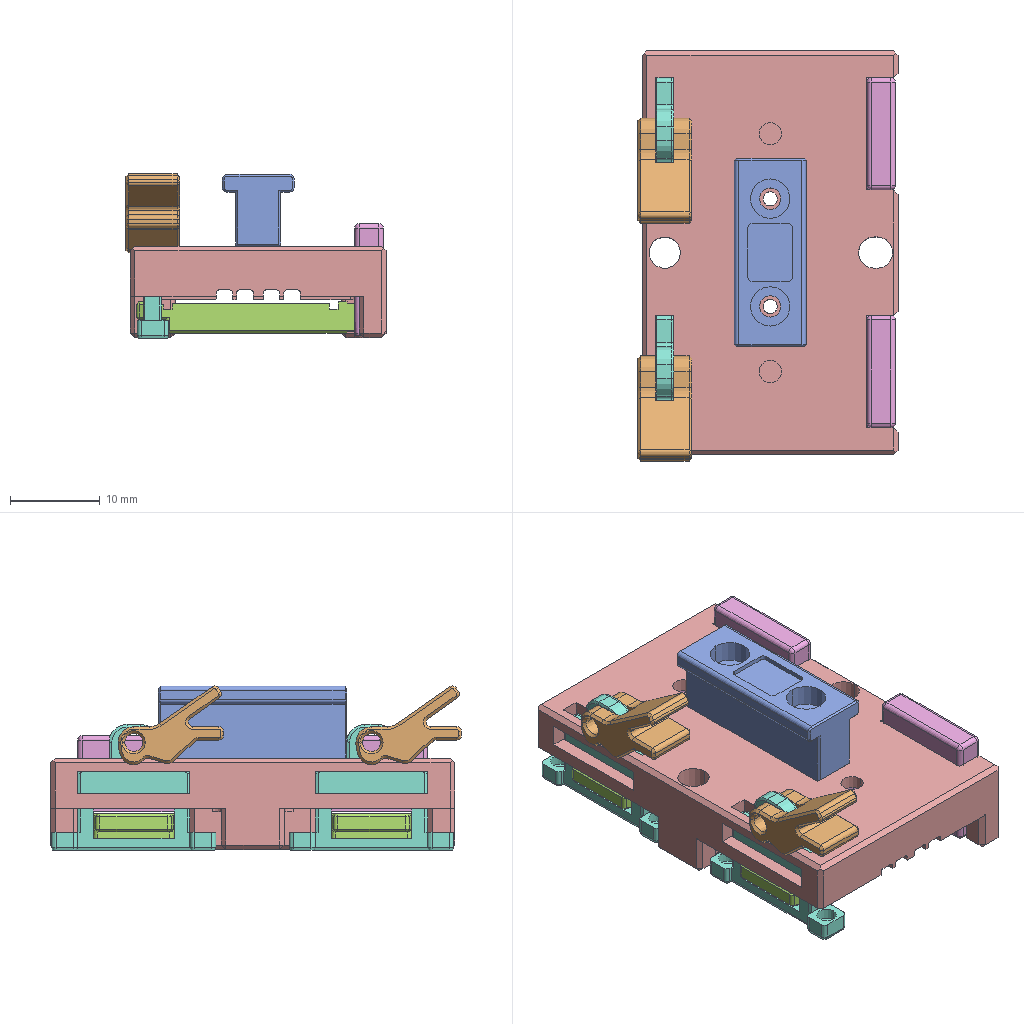Assembly | SolidWorks | 10 different items | 14 placed | box 29 x 46 x 18 mm
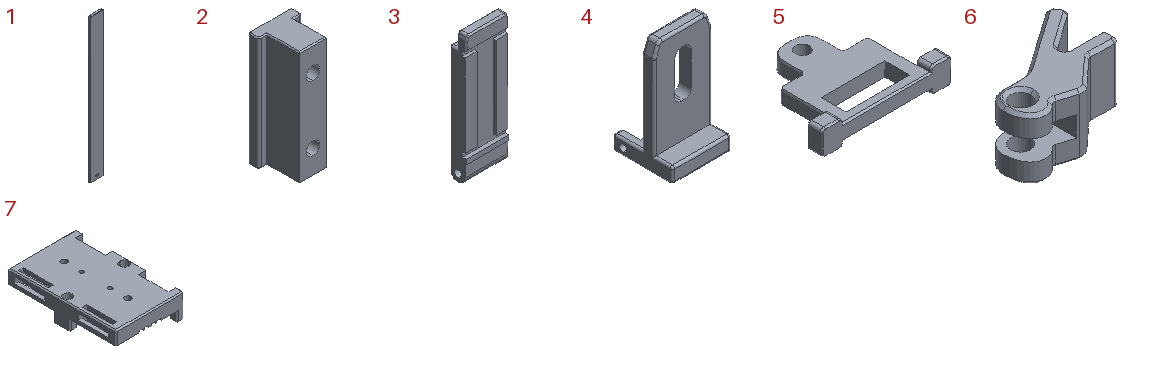Parts list (item | name | quantity | size | volume | features):
1 | - | x1 | 2.9 x 0.45 x 29.5 mm | 37.747 mm3 | features ICE 6, Chamfer 2, Extrusion 1, Fillet 1
2 | - | x1 | 8 x 8 x 21 mm | 820.469 mm3 | features Fillet 2, ICE 2, Chamfer 1, Extrusion 1, HoleWzd 1
3 | - | x2 | 9 x 3.5 x 27.5 mm | 690.682 mm3 | features ICE 6, Chamfer 2, Fillet 2, Extrusion 1
4 | - | x2 | 12.5 x 12.5 x 24 mm | 927.398 mm3 | features ICE 4, Fillet 3, Chamfer 2, Cut 1, Extrusion 1
5 | - | x2 | 18.3 x 14 x 3.5 mm | 236.065 mm3 | features ICE 4, Attribute 3, Fillet 3, Chamfer 1, Extrusion 1, RefAxis 1
6 | - | x2 | 11.75 x 8.783 x 6 mm | 220.036 mm3 | features Attribute 3, ICE 3, Fillet 2, Chamfer 1, Extrusion 1
7 | - | x1 | 28.5 x 45 x 10.2 mm | 4918 mm3 | features ICE 49, Chamfer 5, Fillet 3, HoleWzd 2, Cut 1, DelFace 1, Extrusion 1
8 | JXN-JX01-0597+Latch Retaining Pin | x1 | - | - | -
9 | JXN-JX01-0598+Latch Seat | x1 | - | - | -
10 | Back Side Long Cable Run Simulation | x1 | - | - | -
Mates (type | each side: item.copy, entity, surface, feature):
Width | 7.1 face | 7.1 face | 1.1 face | 1.1 face
Coincident | 7.1 face plane Boss-Extrude1 | 2.1 face plane Boss-Extrude1
Width | 7.1 face plane Boss-Extrude1 | 7.1 face plane Boss-Extrude1 | 2.1 face plane Cut-Extrude1 | 2.1 face plane Cut-Extrude1
Width | 7.1 face plane Boss-Extrude1 | 7.1 face plane Boss-Extrude1 | 2.1 face plane Boss-Extrude1 | 2.1 face plane Boss-Extrude1
Width | 5.1 face plane Boss-Extrude1 | 5.1 face plane Boss-Extrude1 | 7.1 face plane Cut-Extrude1 | 7.1 face plane Cut-Extrude1
Coincident | 7.1 face plane Cut-Extrude71 | 5.1 face plane Boss-Extrude1
Coincident | 5.1 face plane Boss-Extrude1 | 6.1 face plane Cut-Extrude1
Concentric | 5.1 face cylinder Cut-Extrude1 | 6.1 face cylinder Boss-Extrude1
LimitDistanceDim | 5.1 axis | 7.1 face plane Boss-Extrude1
LimitPlanarAngleDim | 7.1 face plane Boss-Extrude1 | 6.1 face plane Boss-Extrude2
Width | 3.1 face plane Boss-Extrude1 | 3.1 face plane Boss-Extrude1 | 5.1 face plane Boss-Extrude1 | 5.1 face plane Boss-Extrude1
Width | 4.1 face plane Boss-Extrude1 | 4.1 face plane Boss-Extrude1 | 7.1 face plane Cut-Extrude1 | 7.1 face plane Cut-Extrude1
Width | 4.1 face plane Boss-Extrude1 | 4.1 face plane Boss-Extrude1 | 7.1 face plane Cut-Extrude66 | 7.1 face plane Cut-Extrude66
Concentric | 3.1 face cylinder Cut-Extrude4 | 4.1 face cylinder Cut-Extrude1
LimitPlanarAngleDim | 4.1 face plane Boss-Extrude1 | 3.1 face plane Boss-Extrude1
LimitDistanceDim | 4.1 face plane Boss-Extrude2 | 7.1 face plane Cut-Extrude78